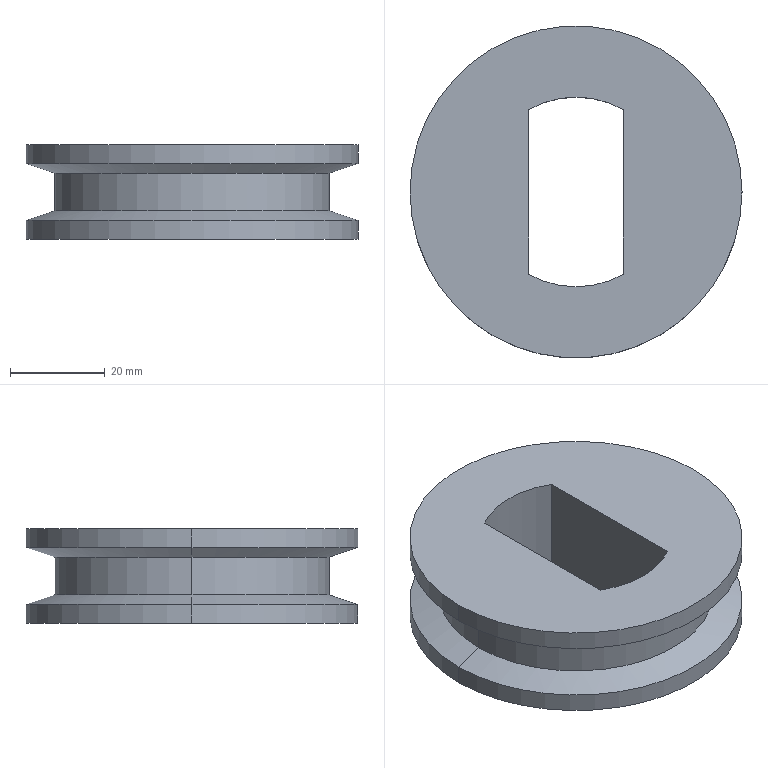Part | SolidWorks | 1 solid | 16 faces | box 70 x 70 x 20 mm | volume 49524 mm3 | cylinder 8 | cone 4 | plane 4 | commonest cylinder face diameters 70 x4 40 x2 58 x2
STEP:
#1=CARTESIAN_POINT('',(35.,0.,10.));
#2=VERTEX_POINT('',#1);
#3=CARTESIAN_POINT('',(-35.,0.,10.));
#4=VERTEX_POINT('',#3);
#5=CARTESIAN_POINT('',(0.,0.,10.));
#6=DIRECTION('',(0.,0.,1.));
#7=DIRECTION('',(1.,0.,0.));
#8=AXIS2_PLACEMENT_3D('',#5,#6,#7);
#9=CIRCLE('',#8,35.);
#10=EDGE_CURVE('',#2,#4,#9,.T.);
#11=ORIENTED_EDGE('',*,*,#10,.F.);
#12=CARTESIAN_POINT('',(35.,0.,6.));
#13=VERTEX_POINT('',#12);
#14=CARTESIAN_POINT('',(35.,0.,10.));
#15=DIRECTION('',(0.,0.,-1.));
#16=VECTOR('',#15,1000.);
#17=LINE('',#14,#16);
#18=EDGE_CURVE('',#2,#13,#17,.T.);
#19=ORIENTED_EDGE('',*,*,#18,.T.);
#20=CARTESIAN_POINT('',(-35.,0.,6.));
#21=VERTEX_POINT('',#20);
#22=CARTESIAN_POINT('',(0.,0.,6.));
#23=DIRECTION('',(0.,0.,-1.));
#24=DIRECTION('',(-1.,0.,0.));
#25=AXIS2_PLACEMENT_3D('',#22,#23,#24);
#26=CIRCLE('',#25,35.);
#27=EDGE_CURVE('',#21,#13,#26,.T.);
#28=ORIENTED_EDGE('',*,*,#27,.F.);
#29=CARTESIAN_POINT('',(-35.,0.,10.));
#30=DIRECTION('',(0.,0.,-1.));
#31=VECTOR('',#30,1000.);
#32=LINE('',#29,#31);
#33=EDGE_CURVE('',#4,#21,#32,.T.);
#34=ORIENTED_EDGE('',*,*,#33,.F.);
#35=EDGE_LOOP('',(#11,#19,#28,#34));
#36=FACE_OUTER_BOUND('',#35,.T.);
#37=CARTESIAN_POINT('',(0.,0.,10.));
#38=DIRECTION('',(0.,0.,-1.));
#39=DIRECTION('',(-1.,0.,0.));
#40=AXIS2_PLACEMENT_3D('',#37,#38,#39);
#41=CYLINDRICAL_SURFACE('',#40,35.);
#42=ADVANCED_FACE('',(#36),#41,.T.);
#43=CARTESIAN_POINT('',(-29.,0.,4.));
#44=VERTEX_POINT('',#43);
#45=CARTESIAN_POINT('',(29.,0.,4.));
#46=VERTEX_POINT('',#45);
#47=CARTESIAN_POINT('',(0.,0.,4.));
#48=DIRECTION('',(0.,0.,-1.));
#49=DIRECTION('',(-1.,0.,0.));
#50=AXIS2_PLACEMENT_3D('',#47,#48,#49);
#51=CIRCLE('',#50,29.);
#52=EDGE_CURVE('',#44,#46,#51,.T.);
#53=ORIENTED_EDGE('',*,*,#52,.F.);
#54=CARTESIAN_POINT('',(-35.,0.,6.));
#55=DIRECTION('',(-0.9487,0.,0.3162));
#56=VECTOR('',#55,1000.);
#57=LINE('',#54,#56);
#58=EDGE_CURVE('',#44,#21,#57,.T.);
#59=ORIENTED_EDGE('',*,*,#58,.T.);
#60=ORIENTED_EDGE('',*,*,#27,.T.);
#61=CARTESIAN_POINT('',(35.,0.,6.));
#62=DIRECTION('',(0.9487,0.,0.3162));
#63=VECTOR('',#62,1000.);
#64=LINE('',#61,#63);
#65=EDGE_CURVE('',#46,#13,#64,.T.);
#66=ORIENTED_EDGE('',*,*,#65,.F.);
#67=EDGE_LOOP('',(#53,#59,#60,#66));
#68=FACE_OUTER_BOUND('',#67,.T.);
#69=CARTESIAN_POINT('',(0.,0.,6.));
#70=DIRECTION('',(0.,0.,1.));
#71=DIRECTION('',(1.,0.,0.));
#72=AXIS2_PLACEMENT_3D('',#69,#70,#71);
#73=CONICAL_SURFACE('',#72,35.,1.249);
#74=ADVANCED_FACE('',(#68),#73,.T.);
#75=ORIENTED_EDGE('',*,*,#52,.T.);
#76=CARTESIAN_POINT('',(29.,0.,-4.));
#77=VERTEX_POINT('',#76);
#78=CARTESIAN_POINT('',(29.,0.,-10.));
#79=DIRECTION('',(0.,0.,-1.));
#80=VECTOR('',#79,1000.);
#81=LINE('',#78,#80);
#82=EDGE_CURVE('',#46,#77,#81,.T.);
#83=ORIENTED_EDGE('',*,*,#82,.T.);
#84=CARTESIAN_POINT('',(-29.,0.,-4.));
#85=VERTEX_POINT('',#84);
#86=CARTESIAN_POINT('',(0.,0.,-4.));
#87=DIRECTION('',(0.,0.,-1.));
#88=DIRECTION('',(-1.,0.,0.));
#89=AXIS2_PLACEMENT_3D('',#86,#87,#88);
#90=CIRCLE('',#89,29.);
#91=EDGE_CURVE('',#85,#77,#90,.T.);
#92=ORIENTED_EDGE('',*,*,#91,.F.);
#93=CARTESIAN_POINT('',(-29.,0.,-10.));
#94=DIRECTION('',(0.,0.,-1.));
#95=VECTOR('',#94,1000.);
#96=LINE('',#93,#95);
#97=EDGE_CURVE('',#44,#85,#96,.T.);
#98=ORIENTED_EDGE('',*,*,#97,.F.);
#99=EDGE_LOOP('',(#75,#83,#92,#98));
#100=FACE_OUTER_BOUND('',#99,.T.);
#101=CARTESIAN_POINT('',(0.,0.,-10.));
#102=DIRECTION('',(0.,0.,-1.));
#103=DIRECTION('',(-1.,0.,0.));
#104=AXIS2_PLACEMENT_3D('',#101,#102,#103);
#105=CYLINDRICAL_SURFACE('',#104,29.);
#106=ADVANCED_FACE('',(#100),#105,.T.);
#107=ORIENTED_EDGE('',*,*,#91,.T.);
#108=CARTESIAN_POINT('',(35.,0.,-6.));
#109=VERTEX_POINT('',#108);
#110=CARTESIAN_POINT('',(29.,0.,-4.));
#111=DIRECTION('',(0.9487,0.,-0.3162));
#112=VECTOR('',#111,1000.);
#113=LINE('',#110,#112);
#114=EDGE_CURVE('',#77,#109,#113,.T.);
#115=ORIENTED_EDGE('',*,*,#114,.T.);
#116=CARTESIAN_POINT('',(-35.,0.,-6.));
#117=VERTEX_POINT('',#116);
#118=CARTESIAN_POINT('',(0.,0.,-6.));
#119=DIRECTION('',(0.,0.,-1.));
#120=DIRECTION('',(-1.,0.,0.));
#121=AXIS2_PLACEMENT_3D('',#118,#119,#120);
#122=CIRCLE('',#121,35.);
#123=EDGE_CURVE('',#117,#109,#122,.T.);
#124=ORIENTED_EDGE('',*,*,#123,.F.);
#125=CARTESIAN_POINT('',(-29.,0.,-4.));
#126=DIRECTION('',(-0.9487,0.,-0.3162));
#127=VECTOR('',#126,1000.);
#128=LINE('',#125,#127);
#129=EDGE_CURVE('',#85,#117,#128,.T.);
#130=ORIENTED_EDGE('',*,*,#129,.F.);
#131=EDGE_LOOP('',(#107,#115,#124,#130));
#132=FACE_OUTER_BOUND('',#131,.T.);
#133=CARTESIAN_POINT('',(0.,0.,-4.));
#134=DIRECTION('',(0.,0.,-1.));
#135=DIRECTION('',(-1.,0.,0.));
#136=AXIS2_PLACEMENT_3D('',#133,#134,#135);
#137=CONICAL_SURFACE('',#136,29.,1.249);
#138=ADVANCED_FACE('',(#132),#137,.T.);
#139=ORIENTED_EDGE('',*,*,#123,.T.);
#140=CARTESIAN_POINT('',(35.,0.,-10.));
#141=VERTEX_POINT('',#140);
#142=CARTESIAN_POINT('',(35.,0.,10.));
#143=DIRECTION('',(0.,0.,-1.));
#144=VECTOR('',#143,1000.);
#145=LINE('',#142,#144);
#146=EDGE_CURVE('',#109,#141,#145,.T.);
#147=ORIENTED_EDGE('',*,*,#146,.T.);
#148=CARTESIAN_POINT('',(-35.,0.,-10.));
#149=VERTEX_POINT('',#148);
#150=CARTESIAN_POINT('',(0.,0.,-10.));
#151=DIRECTION('',(0.,0.,1.));
#152=DIRECTION('',(1.,0.,0.));
#153=AXIS2_PLACEMENT_3D('',#150,#151,#152);
#154=CIRCLE('',#153,35.);
#155=EDGE_CURVE('',#141,#149,#154,.T.);
#156=ORIENTED_EDGE('',*,*,#155,.T.);
#157=CARTESIAN_POINT('',(-35.,0.,10.));
#158=DIRECTION('',(0.,0.,-1.));
#159=VECTOR('',#158,1000.);
#160=LINE('',#157,#159);
#161=EDGE_CURVE('',#117,#149,#160,.T.);
#162=ORIENTED_EDGE('',*,*,#161,.F.);
#163=EDGE_LOOP('',(#139,#147,#156,#162));
#164=FACE_OUTER_BOUND('',#163,.T.);
#165=CARTESIAN_POINT('',(0.,0.,10.));
#166=DIRECTION('',(0.,0.,-1.));
#167=DIRECTION('',(-1.,0.,0.));
#168=AXIS2_PLACEMENT_3D('',#165,#166,#167);
#169=CYLINDRICAL_SURFACE('',#168,35.);
#170=ADVANCED_FACE('',(#164),#169,.T.);
#171=ORIENTED_EDGE('',*,*,#146,.F.);
#172=CARTESIAN_POINT('',(0.,0.,-6.));
#173=DIRECTION('',(0.,0.,-1.));
#174=DIRECTION('',(-1.,0.,0.));
#175=AXIS2_PLACEMENT_3D('',#172,#173,#174);
#176=CIRCLE('',#175,35.);
#177=EDGE_CURVE('',#109,#117,#176,.T.);
#178=ORIENTED_EDGE('',*,*,#177,.T.);
#179=ORIENTED_EDGE('',*,*,#161,.T.);
#180=CARTESIAN_POINT('',(0.,0.,-10.));
#181=DIRECTION('',(0.,0.,1.));
#182=DIRECTION('',(1.,0.,0.));
#183=AXIS2_PLACEMENT_3D('',#180,#181,#182);
#184=CIRCLE('',#183,35.);
#185=EDGE_CURVE('',#149,#141,#184,.T.);
#186=ORIENTED_EDGE('',*,*,#185,.T.);
#187=EDGE_LOOP('',(#171,#178,#179,#186));
#188=FACE_OUTER_BOUND('',#187,.T.);
#189=CARTESIAN_POINT('',(0.,0.,10.));
#190=DIRECTION('',(0.,0.,-1.));
#191=DIRECTION('',(-1.,0.,0.));
#192=AXIS2_PLACEMENT_3D('',#189,#190,#191);
#193=CYLINDRICAL_SURFACE('',#192,35.);
#194=ADVANCED_FACE('',(#188),#193,.T.);
#195=CARTESIAN_POINT('',(10.,17.321,-10.));
#196=VERTEX_POINT('',#195);
#197=CARTESIAN_POINT('',(10.,-17.321,-10.));
#198=VERTEX_POINT('',#197);
#199=CARTESIAN_POINT('',(10.,0.,-10.));
#200=DIRECTION('',(0.,-1.,0.));
#201=VECTOR('',#200,1000.);
#202=LINE('',#199,#201);
#203=EDGE_CURVE('',#196,#198,#202,.T.);
#204=ORIENTED_EDGE('',*,*,#203,.F.);
#205=CARTESIAN_POINT('',(-10.,17.321,-10.));
#206=VERTEX_POINT('',#205);
#207=CARTESIAN_POINT('',(0.,0.,-10.));
#208=DIRECTION('',(0.,0.,-1.));
#209=DIRECTION('',(-1.,0.,0.));
#210=AXIS2_PLACEMENT_3D('',#207,#208,#209);
#211=CIRCLE('',#210,20.);
#212=EDGE_CURVE('',#206,#196,#211,.T.);
#213=ORIENTED_EDGE('',*,*,#212,.F.);
#214=CARTESIAN_POINT('',(-10.,-17.321,-10.));
#215=VERTEX_POINT('',#214);
#216=CARTESIAN_POINT('',(-10.,0.,-10.));
#217=DIRECTION('',(0.,-1.,0.));
#218=VECTOR('',#217,1000.);
#219=LINE('',#216,#218);
#220=EDGE_CURVE('',#206,#215,#219,.T.);
#221=ORIENTED_EDGE('',*,*,#220,.T.);
#222=CARTESIAN_POINT('',(0.,0.,-10.));
#223=DIRECTION('',(0.,0.,-1.));
#224=DIRECTION('',(-1.,0.,0.));
#225=AXIS2_PLACEMENT_3D('',#222,#223,#224);
#226=CIRCLE('',#225,20.);
#227=EDGE_CURVE('',#198,#215,#226,.T.);
#228=ORIENTED_EDGE('',*,*,#227,.F.);
#229=EDGE_LOOP('',(#204,#213,#221,#228));
#230=FACE_BOUND('',#229,.T.);
#231=ORIENTED_EDGE('',*,*,#185,.F.);
#232=ORIENTED_EDGE('',*,*,#155,.F.);
#233=EDGE_LOOP('',(#231,#232));
#234=FACE_OUTER_BOUND('',#233,.T.);
#235=CARTESIAN_POINT('',(0.,0.,-10.));
#236=DIRECTION('',(0.,0.,1.));
#237=DIRECTION('',(1.,0.,0.));
#238=AXIS2_PLACEMENT_3D('',#235,#236,#237);
#239=PLANE('',#238);
#240=ADVANCED_FACE('',(#230,#234),#239,.F.);
#241=ORIENTED_EDGE('',*,*,#114,.F.);
#242=CARTESIAN_POINT('',(0.,0.,-4.));
#243=DIRECTION('',(0.,0.,-1.));
#244=DIRECTION('',(-1.,0.,0.));
#245=AXIS2_PLACEMENT_3D('',#242,#243,#244);
#246=CIRCLE('',#245,29.);
#247=EDGE_CURVE('',#77,#85,#246,.T.);
#248=ORIENTED_EDGE('',*,*,#247,.T.);
#249=ORIENTED_EDGE('',*,*,#129,.T.);
#250=ORIENTED_EDGE('',*,*,#177,.F.);
#251=EDGE_LOOP('',(#241,#248,#249,#250));
#252=FACE_OUTER_BOUND('',#251,.T.);
#253=CARTESIAN_POINT('',(0.,0.,-4.));
#254=DIRECTION('',(0.,0.,-1.));
#255=DIRECTION('',(-1.,0.,0.));
#256=AXIS2_PLACEMENT_3D('',#253,#254,#255);
#257=CONICAL_SURFACE('',#256,29.,1.249);
#258=ADVANCED_FACE('',(#252),#257,.T.);
#259=ORIENTED_EDGE('',*,*,#82,.F.);
#260=CARTESIAN_POINT('',(0.,0.,4.));
#261=DIRECTION('',(0.,0.,-1.));
#262=DIRECTION('',(-1.,0.,0.));
#263=AXIS2_PLACEMENT_3D('',#260,#261,#262);
#264=CIRCLE('',#263,29.);
#265=EDGE_CURVE('',#46,#44,#264,.T.);
#266=ORIENTED_EDGE('',*,*,#265,.T.);
#267=ORIENTED_EDGE('',*,*,#97,.T.);
#268=ORIENTED_EDGE('',*,*,#247,.F.);
#269=EDGE_LOOP('',(#259,#266,#267,#268));
#270=FACE_OUTER_BOUND('',#269,.T.);
#271=CARTESIAN_POINT('',(0.,0.,-10.));
#272=DIRECTION('',(0.,0.,-1.));
#273=DIRECTION('',(-1.,0.,0.));
#274=AXIS2_PLACEMENT_3D('',#271,#272,#273);
#275=CYLINDRICAL_SURFACE('',#274,29.);
#276=ADVANCED_FACE('',(#270),#275,.T.);
#277=ORIENTED_EDGE('',*,*,#58,.F.);
#278=ORIENTED_EDGE('',*,*,#265,.F.);
#279=ORIENTED_EDGE('',*,*,#65,.T.);
#280=CARTESIAN_POINT('',(0.,0.,6.));
#281=DIRECTION('',(0.,0.,-1.));
#282=DIRECTION('',(-1.,0.,0.));
#283=AXIS2_PLACEMENT_3D('',#280,#281,#282);
#284=CIRCLE('',#283,35.);
#285=EDGE_CURVE('',#13,#21,#284,.T.);
#286=ORIENTED_EDGE('',*,*,#285,.T.);
#287=EDGE_LOOP('',(#277,#278,#279,#286));
#288=FACE_OUTER_BOUND('',#287,.T.);
#289=CARTESIAN_POINT('',(0.,0.,6.));
#290=DIRECTION('',(0.,0.,1.));
#291=DIRECTION('',(1.,0.,0.));
#292=AXIS2_PLACEMENT_3D('',#289,#290,#291);
#293=CONICAL_SURFACE('',#292,35.,1.249);
#294=ADVANCED_FACE('',(#288),#293,.T.);
#295=CARTESIAN_POINT('',(-10.,17.321,10.));
#296=VERTEX_POINT('',#295);
#297=CARTESIAN_POINT('',(10.,17.321,10.));
#298=VERTEX_POINT('',#297);
#299=CARTESIAN_POINT('',(0.,0.,10.));
#300=DIRECTION('',(0.,0.,-1.));
#301=DIRECTION('',(-1.,0.,0.));
#302=AXIS2_PLACEMENT_3D('',#299,#300,#301);
#303=CIRCLE('',#302,20.);
#304=EDGE_CURVE('',#296,#298,#303,.T.);
#305=ORIENTED_EDGE('',*,*,#304,.T.);
#306=CARTESIAN_POINT('',(10.,-17.321,10.));
#307=VERTEX_POINT('',#306);
#308=CARTESIAN_POINT('',(10.,0.,10.));
#309=DIRECTION('',(0.,-1.,0.));
#310=VECTOR('',#309,1000.);
#311=LINE('',#308,#310);
#312=EDGE_CURVE('',#298,#307,#311,.T.);
#313=ORIENTED_EDGE('',*,*,#312,.T.);
#314=CARTESIAN_POINT('',(-10.,-17.321,10.));
#315=VERTEX_POINT('',#314);
#316=CARTESIAN_POINT('',(0.,0.,10.));
#317=DIRECTION('',(0.,0.,-1.));
#318=DIRECTION('',(-1.,0.,0.));
#319=AXIS2_PLACEMENT_3D('',#316,#317,#318);
#320=CIRCLE('',#319,20.);
#321=EDGE_CURVE('',#307,#315,#320,.T.);
#322=ORIENTED_EDGE('',*,*,#321,.T.);
#323=CARTESIAN_POINT('',(-10.,0.,10.));
#324=DIRECTION('',(0.,-1.,0.));
#325=VECTOR('',#324,1000.);
#326=LINE('',#323,#325);
#327=EDGE_CURVE('',#296,#315,#326,.T.);
#328=ORIENTED_EDGE('',*,*,#327,.F.);
#329=EDGE_LOOP('',(#305,#313,#322,#328));
#330=FACE_BOUND('',#329,.T.);
#331=CARTESIAN_POINT('',(0.,0.,10.));
#332=DIRECTION('',(0.,0.,1.));
#333=DIRECTION('',(1.,0.,0.));
#334=AXIS2_PLACEMENT_3D('',#331,#332,#333);
#335=CIRCLE('',#334,35.);
#336=EDGE_CURVE('',#4,#2,#335,.T.);
#337=ORIENTED_EDGE('',*,*,#336,.T.);
#338=ORIENTED_EDGE('',*,*,#10,.T.);
#339=EDGE_LOOP('',(#337,#338));
#340=FACE_OUTER_BOUND('',#339,.T.);
#341=CARTESIAN_POINT('',(0.,0.,10.));
#342=DIRECTION('',(0.,0.,1.));
#343=DIRECTION('',(1.,0.,0.));
#344=AXIS2_PLACEMENT_3D('',#341,#342,#343);
#345=PLANE('',#344);
#346=ADVANCED_FACE('',(#330,#340),#345,.T.);
#347=ORIENTED_EDGE('',*,*,#18,.F.);
#348=ORIENTED_EDGE('',*,*,#336,.F.);
#349=ORIENTED_EDGE('',*,*,#33,.T.);
#350=ORIENTED_EDGE('',*,*,#285,.F.);
#351=EDGE_LOOP('',(#347,#348,#349,#350));
#352=FACE_OUTER_BOUND('',#351,.T.);
#353=CARTESIAN_POINT('',(0.,0.,10.));
#354=DIRECTION('',(0.,0.,-1.));
#355=DIRECTION('',(-1.,0.,0.));
#356=AXIS2_PLACEMENT_3D('',#353,#354,#355);
#357=CYLINDRICAL_SURFACE('',#356,35.);
#358=ADVANCED_FACE('',(#352),#357,.T.);
#359=ORIENTED_EDGE('',*,*,#212,.T.);
#360=CARTESIAN_POINT('',(10.,17.321,10.));
#361=DIRECTION('',(0.,0.,-1.));
#362=VECTOR('',#361,1000.);
#363=LINE('',#360,#362);
#364=EDGE_CURVE('',#298,#196,#363,.T.);
#365=ORIENTED_EDGE('',*,*,#364,.F.);
#366=ORIENTED_EDGE('',*,*,#304,.F.);
#367=CARTESIAN_POINT('',(-10.,17.321,10.));
#368=DIRECTION('',(0.,0.,-1.));
#369=VECTOR('',#368,1000.);
#370=LINE('',#367,#369);
#371=EDGE_CURVE('',#296,#206,#370,.T.);
#372=ORIENTED_EDGE('',*,*,#371,.T.);
#373=EDGE_LOOP('',(#359,#365,#366,#372));
#374=FACE_OUTER_BOUND('',#373,.T.);
#375=CARTESIAN_POINT('',(0.,0.,10.));
#376=DIRECTION('',(0.,0.,-1.));
#377=DIRECTION('',(-1.,0.,0.));
#378=AXIS2_PLACEMENT_3D('',#375,#376,#377);
#379=CYLINDRICAL_SURFACE('',#378,20.);
#380=ADVANCED_FACE('',(#374),#379,.F.);
#381=ORIENTED_EDGE('',*,*,#220,.F.);
#382=ORIENTED_EDGE('',*,*,#371,.F.);
#383=ORIENTED_EDGE('',*,*,#327,.T.);
#384=CARTESIAN_POINT('',(-10.,-17.321,10.));
#385=DIRECTION('',(0.,0.,-1.));
#386=VECTOR('',#385,1000.);
#387=LINE('',#384,#386);
#388=EDGE_CURVE('',#315,#215,#387,.T.);
#389=ORIENTED_EDGE('',*,*,#388,.T.);
#390=EDGE_LOOP('',(#381,#382,#383,#389));
#391=FACE_OUTER_BOUND('',#390,.T.);
#392=CARTESIAN_POINT('',(-10.,0.,10.));
#393=DIRECTION('',(1.,0.,0.));
#394=DIRECTION('',(0.,0.,-1.));
#395=AXIS2_PLACEMENT_3D('',#392,#393,#394);
#396=PLANE('',#395);
#397=ADVANCED_FACE('',(#391),#396,.T.);
#398=ORIENTED_EDGE('',*,*,#227,.T.);
#399=ORIENTED_EDGE('',*,*,#388,.F.);
#400=ORIENTED_EDGE('',*,*,#321,.F.);
#401=CARTESIAN_POINT('',(10.,-17.321,10.));
#402=DIRECTION('',(0.,0.,-1.));
#403=VECTOR('',#402,1000.);
#404=LINE('',#401,#403);
#405=EDGE_CURVE('',#307,#198,#404,.T.);
#406=ORIENTED_EDGE('',*,*,#405,.T.);
#407=EDGE_LOOP('',(#398,#399,#400,#406));
#408=FACE_OUTER_BOUND('',#407,.T.);
#409=CARTESIAN_POINT('',(0.,0.,10.));
#410=DIRECTION('',(0.,0.,-1.));
#411=DIRECTION('',(-1.,0.,0.));
#412=AXIS2_PLACEMENT_3D('',#409,#410,#411);
#413=CYLINDRICAL_SURFACE('',#412,20.);
#414=ADVANCED_FACE('',(#408),#413,.F.);
#415=ORIENTED_EDGE('',*,*,#203,.T.);
#416=ORIENTED_EDGE('',*,*,#405,.F.);
#417=ORIENTED_EDGE('',*,*,#312,.F.);
#418=ORIENTED_EDGE('',*,*,#364,.T.);
#419=EDGE_LOOP('',(#415,#416,#417,#418));
#420=FACE_OUTER_BOUND('',#419,.T.);
#421=CARTESIAN_POINT('',(10.,0.,10.));
#422=DIRECTION('',(1.,0.,0.));
#423=DIRECTION('',(0.,0.,-1.));
#424=AXIS2_PLACEMENT_3D('',#421,#422,#423);
#425=PLANE('',#424);
#426=ADVANCED_FACE('',(#420),#425,.F.);
#427=CLOSED_SHELL('',(#42,#74,#106,#138,#170,#194,#240,#258,#276,#294,#346,#358,#380,#397,#414,#426));
#428=MANIFOLD_SOLID_BREP('',#427);
#429=CARTESIAN_POINT('',(0.,0.,0.));
#430=DIRECTION('',(0.,0.,1.));
#431=DIRECTION('',(1.,0.,0.));
#432=AXIS2_PLACEMENT_3D('',#429,#430,#431);
#433=(LENGTH_UNIT()NAMED_UNIT(*)SI_UNIT(.MILLI.,.METRE.));
#434=UNCERTAINTY_MEASURE_WITH_UNIT(LENGTH_MEASURE(0.00001),#433,'','');
#435=(NAMED_UNIT(*)PLANE_ANGLE_UNIT()SI_UNIT($,.RADIAN.));
#436=(NAMED_UNIT(*)SI_UNIT($,.STERADIAN.)SOLID_ANGLE_UNIT());
#437=(GEOMETRIC_REPRESENTATION_CONTEXT(3)GLOBAL_UNCERTAINTY_ASSIGNED_CONTEXT((#434))GLOBAL_UNIT_ASSIGNED_CONTEXT((#433,#435,#436))REPRESENTATION_CONTEXT('',''));
#438=ADVANCED_BREP_SHAPE_REPRESENTATION('',(#428,#432),#437);